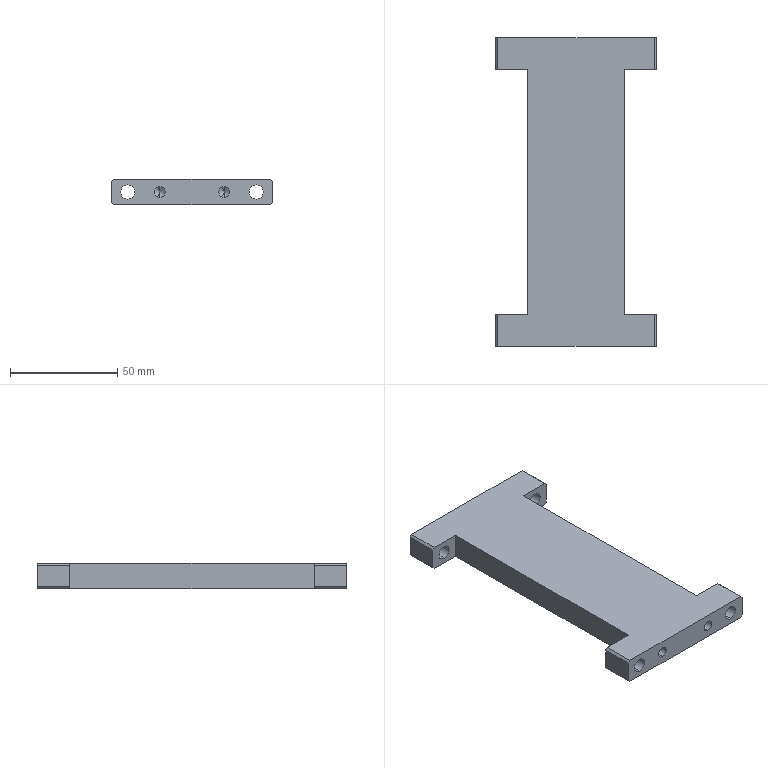Part | SolidWorks | features HoleWzd 2, MirrorPattern 2, Chamfer 1, Extrusion 1, ICE 1 | 1 solid | 46 faces | box 75 x 144 x 12 mm | volume 85544 mm3 | plane 22 | cylinder 16 | cone 8 | commonest cylinder face diameters 5 x8 6.6 x8
STEP:
#1=CARTESIAN_POINT('',(15.,61.,-2.5));
#2=VERTEX_POINT('',#1);
#3=CARTESIAN_POINT('',(15.,61.,2.5));
#4=VERTEX_POINT('',#3);
#5=CARTESIAN_POINT('',(15.,61.,0.));
#6=DIRECTION('',(0.,1.,0.));
#7=DIRECTION('',(0.,0.,1.));
#8=AXIS2_PLACEMENT_3D('',#5,#6,#7);
#9=CIRCLE('',#8,2.5);
#10=EDGE_CURVE('',#2,#4,#9,.T.);
#11=ORIENTED_EDGE('',*,*,#10,.F.);
#12=CARTESIAN_POINT('',(15.,72.,-2.5));
#13=VERTEX_POINT('',#12);
#14=CARTESIAN_POINT('',(15.,72.,-2.5));
#15=DIRECTION('',(0.,1.,0.));
#16=VECTOR('',#15,1000.);
#17=LINE('',#14,#16);
#18=EDGE_CURVE('',#2,#13,#17,.T.);
#19=ORIENTED_EDGE('',*,*,#18,.T.);
#20=CARTESIAN_POINT('',(15.,72.,2.5));
#21=VERTEX_POINT('',#20);
#22=CARTESIAN_POINT('',(15.,72.,0.));
#23=DIRECTION('',(0.,1.,0.));
#24=DIRECTION('',(0.,0.,1.));
#25=AXIS2_PLACEMENT_3D('',#22,#23,#24);
#26=CIRCLE('',#25,2.5);
#27=EDGE_CURVE('',#13,#21,#26,.T.);
#28=ORIENTED_EDGE('',*,*,#27,.T.);
#29=CARTESIAN_POINT('',(15.,72.,2.5));
#30=DIRECTION('',(0.,1.,0.));
#31=VECTOR('',#30,1000.);
#32=LINE('',#29,#31);
#33=EDGE_CURVE('',#4,#21,#32,.T.);
#34=ORIENTED_EDGE('',*,*,#33,.F.);
#35=EDGE_LOOP('',(#11,#19,#28,#34));
#36=FACE_OUTER_BOUND('',#35,.T.);
#37=CARTESIAN_POINT('',(15.,72.,0.));
#38=DIRECTION('',(0.,1.,0.));
#39=DIRECTION('',(0.,0.,1.));
#40=AXIS2_PLACEMENT_3D('',#37,#38,#39);
#41=CYLINDRICAL_SURFACE('',#40,2.5);
#42=ADVANCED_FACE('',(#36),#41,.F.);
#43=CARTESIAN_POINT('',(15.,59.498,0.));
#44=VERTEX_POINT('',#43);
#45=CARTESIAN_POINT('',(15.,61.,2.5));
#46=DIRECTION('',(0.,0.515,0.8572));
#47=VECTOR('',#46,1000.);
#48=LINE('',#45,#47);
#49=EDGE_CURVE('',#44,#4,#48,.T.);
#50=ORIENTED_EDGE('',*,*,#49,.F.);
#51=CARTESIAN_POINT('',(15.,61.,-2.5));
#52=DIRECTION('',(0.,0.515,-0.8572));
#53=VECTOR('',#52,1000.);
#54=LINE('',#51,#53);
#55=EDGE_CURVE('',#44,#2,#54,.T.);
#56=ORIENTED_EDGE('',*,*,#55,.T.);
#57=ORIENTED_EDGE('',*,*,#10,.T.);
#58=EDGE_LOOP('',(#50,#56,#57));
#59=FACE_OUTER_BOUND('',#58,.T.);
#60=CARTESIAN_POINT('',(15.,61.,0.));
#61=DIRECTION('',(0.,1.,0.));
#62=DIRECTION('',(0.,0.,1.));
#63=AXIS2_PLACEMENT_3D('',#60,#61,#62);
#64=CONICAL_SURFACE('',#63,2.5,1.03);
#65=ADVANCED_FACE('',(#59),#64,.F.);
#66=CARTESIAN_POINT('',(-15.,61.,-2.5));
#67=VERTEX_POINT('',#66);
#68=CARTESIAN_POINT('',(-15.,61.,2.5));
#69=VERTEX_POINT('',#68);
#70=CARTESIAN_POINT('',(-15.,61.,0.));
#71=DIRECTION('',(0.,1.,0.));
#72=DIRECTION('',(0.,0.,1.));
#73=AXIS2_PLACEMENT_3D('',#70,#71,#72);
#74=CIRCLE('',#73,2.5);
#75=EDGE_CURVE('',#67,#69,#74,.T.);
#76=ORIENTED_EDGE('',*,*,#75,.F.);
#77=CARTESIAN_POINT('',(-15.,72.,-2.5));
#78=VERTEX_POINT('',#77);
#79=CARTESIAN_POINT('',(-15.,72.,-2.5));
#80=DIRECTION('',(0.,1.,0.));
#81=VECTOR('',#80,1000.);
#82=LINE('',#79,#81);
#83=EDGE_CURVE('',#67,#78,#82,.T.);
#84=ORIENTED_EDGE('',*,*,#83,.T.);
#85=CARTESIAN_POINT('',(-15.,72.,2.5));
#86=VERTEX_POINT('',#85);
#87=CARTESIAN_POINT('',(-15.,72.,0.));
#88=DIRECTION('',(0.,1.,0.));
#89=DIRECTION('',(0.,0.,1.));
#90=AXIS2_PLACEMENT_3D('',#87,#88,#89);
#91=CIRCLE('',#90,2.5);
#92=EDGE_CURVE('',#78,#86,#91,.T.);
#93=ORIENTED_EDGE('',*,*,#92,.T.);
#94=CARTESIAN_POINT('',(-15.,72.,2.5));
#95=DIRECTION('',(0.,1.,0.));
#96=VECTOR('',#95,1000.);
#97=LINE('',#94,#96);
#98=EDGE_CURVE('',#69,#86,#97,.T.);
#99=ORIENTED_EDGE('',*,*,#98,.F.);
#100=EDGE_LOOP('',(#76,#84,#93,#99));
#101=FACE_OUTER_BOUND('',#100,.T.);
#102=CARTESIAN_POINT('',(-15.,72.,0.));
#103=DIRECTION('',(0.,1.,0.));
#104=DIRECTION('',(0.,0.,1.));
#105=AXIS2_PLACEMENT_3D('',#102,#103,#104);
#106=CYLINDRICAL_SURFACE('',#105,2.5);
#107=ADVANCED_FACE('',(#101),#106,.F.);
#108=CARTESIAN_POINT('',(-15.,59.498,0.));
#109=VERTEX_POINT('',#108);
#110=CARTESIAN_POINT('',(-15.,61.,2.5));
#111=DIRECTION('',(0.,0.515,0.8572));
#112=VECTOR('',#111,1000.);
#113=LINE('',#110,#112);
#114=EDGE_CURVE('',#109,#69,#113,.T.);
#115=ORIENTED_EDGE('',*,*,#114,.F.);
#116=CARTESIAN_POINT('',(-15.,61.,-2.5));
#117=DIRECTION('',(0.,0.515,-0.8572));
#118=VECTOR('',#117,1000.);
#119=LINE('',#116,#118);
#120=EDGE_CURVE('',#109,#67,#119,.T.);
#121=ORIENTED_EDGE('',*,*,#120,.T.);
#122=ORIENTED_EDGE('',*,*,#75,.T.);
#123=EDGE_LOOP('',(#115,#121,#122));
#124=FACE_OUTER_BOUND('',#123,.T.);
#125=CARTESIAN_POINT('',(-15.,61.,0.));
#126=DIRECTION('',(0.,1.,0.));
#127=DIRECTION('',(0.,0.,1.));
#128=AXIS2_PLACEMENT_3D('',#125,#126,#127);
#129=CONICAL_SURFACE('',#128,2.5,1.03);
#130=ADVANCED_FACE('',(#124),#129,.F.);
#131=CARTESIAN_POINT('',(15.,-61.,2.5));
#132=VERTEX_POINT('',#131);
#133=CARTESIAN_POINT('',(15.,-61.,-2.5));
#134=VERTEX_POINT('',#133);
#135=CARTESIAN_POINT('',(15.,-61.,0.));
#136=DIRECTION('',(0.,-1.,0.));
#137=DIRECTION('',(0.,0.,-1.));
#138=AXIS2_PLACEMENT_3D('',#135,#136,#137);
#139=CIRCLE('',#138,2.5);
#140=EDGE_CURVE('',#132,#134,#139,.T.);
#141=ORIENTED_EDGE('',*,*,#140,.F.);
#142=CARTESIAN_POINT('',(15.,-72.,2.5));
#143=VERTEX_POINT('',#142);
#144=CARTESIAN_POINT('',(15.,-72.,2.5));
#145=DIRECTION('',(0.,-1.,0.));
#146=VECTOR('',#145,1000.);
#147=LINE('',#144,#146);
#148=EDGE_CURVE('',#132,#143,#147,.T.);
#149=ORIENTED_EDGE('',*,*,#148,.T.);
#150=CARTESIAN_POINT('',(15.,-72.,-2.5));
#151=VERTEX_POINT('',#150);
#152=CARTESIAN_POINT('',(15.,-72.,0.));
#153=DIRECTION('',(0.,-1.,0.));
#154=DIRECTION('',(0.,0.,-1.));
#155=AXIS2_PLACEMENT_3D('',#152,#153,#154);
#156=CIRCLE('',#155,2.5);
#157=EDGE_CURVE('',#143,#151,#156,.T.);
#158=ORIENTED_EDGE('',*,*,#157,.T.);
#159=CARTESIAN_POINT('',(15.,-72.,-2.5));
#160=DIRECTION('',(0.,-1.,0.));
#161=VECTOR('',#160,1000.);
#162=LINE('',#159,#161);
#163=EDGE_CURVE('',#134,#151,#162,.T.);
#164=ORIENTED_EDGE('',*,*,#163,.F.);
#165=EDGE_LOOP('',(#141,#149,#158,#164));
#166=FACE_OUTER_BOUND('',#165,.T.);
#167=CARTESIAN_POINT('',(15.,-72.,0.));
#168=DIRECTION('',(0.,-1.,0.));
#169=DIRECTION('',(0.,0.,-1.));
#170=AXIS2_PLACEMENT_3D('',#167,#168,#169);
#171=CYLINDRICAL_SURFACE('',#170,2.5);
#172=ADVANCED_FACE('',(#166),#171,.F.);
#173=CARTESIAN_POINT('',(15.,-59.498,0.));
#174=VERTEX_POINT('',#173);
#175=CARTESIAN_POINT('',(15.,-61.,-2.5));
#176=DIRECTION('',(0.,-0.515,-0.8572));
#177=VECTOR('',#176,1000.);
#178=LINE('',#175,#177);
#179=EDGE_CURVE('',#174,#134,#178,.T.);
#180=ORIENTED_EDGE('',*,*,#179,.F.);
#181=CARTESIAN_POINT('',(15.,-61.,2.5));
#182=DIRECTION('',(0.,-0.515,0.8572));
#183=VECTOR('',#182,1000.);
#184=LINE('',#181,#183);
#185=EDGE_CURVE('',#174,#132,#184,.T.);
#186=ORIENTED_EDGE('',*,*,#185,.T.);
#187=ORIENTED_EDGE('',*,*,#140,.T.);
#188=EDGE_LOOP('',(#180,#186,#187));
#189=FACE_OUTER_BOUND('',#188,.T.);
#190=CARTESIAN_POINT('',(15.,-61.,0.));
#191=DIRECTION('',(0.,-1.,0.));
#192=DIRECTION('',(0.,0.,-1.));
#193=AXIS2_PLACEMENT_3D('',#190,#191,#192);
#194=CONICAL_SURFACE('',#193,2.5,1.03);
#195=ADVANCED_FACE('',(#189),#194,.F.);
#196=CARTESIAN_POINT('',(-15.,-61.,2.5));
#197=VERTEX_POINT('',#196);
#198=CARTESIAN_POINT('',(-15.,-61.,-2.5));
#199=VERTEX_POINT('',#198);
#200=CARTESIAN_POINT('',(-15.,-61.,0.));
#201=DIRECTION('',(0.,-1.,0.));
#202=DIRECTION('',(0.,0.,-1.));
#203=AXIS2_PLACEMENT_3D('',#200,#201,#202);
#204=CIRCLE('',#203,2.5);
#205=EDGE_CURVE('',#197,#199,#204,.T.);
#206=ORIENTED_EDGE('',*,*,#205,.F.);
#207=CARTESIAN_POINT('',(-15.,-72.,2.5));
#208=VERTEX_POINT('',#207);
#209=CARTESIAN_POINT('',(-15.,-72.,2.5));
#210=DIRECTION('',(0.,-1.,0.));
#211=VECTOR('',#210,1000.);
#212=LINE('',#209,#211);
#213=EDGE_CURVE('',#197,#208,#212,.T.);
#214=ORIENTED_EDGE('',*,*,#213,.T.);
#215=CARTESIAN_POINT('',(-15.,-72.,-2.5));
#216=VERTEX_POINT('',#215);
#217=CARTESIAN_POINT('',(-15.,-72.,0.));
#218=DIRECTION('',(0.,-1.,0.));
#219=DIRECTION('',(0.,0.,-1.));
#220=AXIS2_PLACEMENT_3D('',#217,#218,#219);
#221=CIRCLE('',#220,2.5);
#222=EDGE_CURVE('',#208,#216,#221,.T.);
#223=ORIENTED_EDGE('',*,*,#222,.T.);
#224=CARTESIAN_POINT('',(-15.,-72.,-2.5));
#225=DIRECTION('',(0.,-1.,0.));
#226=VECTOR('',#225,1000.);
#227=LINE('',#224,#226);
#228=EDGE_CURVE('',#199,#216,#227,.T.);
#229=ORIENTED_EDGE('',*,*,#228,.F.);
#230=EDGE_LOOP('',(#206,#214,#223,#229));
#231=FACE_OUTER_BOUND('',#230,.T.);
#232=CARTESIAN_POINT('',(-15.,-72.,0.));
#233=DIRECTION('',(0.,-1.,0.));
#234=DIRECTION('',(0.,0.,-1.));
#235=AXIS2_PLACEMENT_3D('',#232,#233,#234);
#236=CYLINDRICAL_SURFACE('',#235,2.5);
#237=ADVANCED_FACE('',(#231),#236,.F.);
#238=CARTESIAN_POINT('',(-15.,-59.498,0.));
#239=VERTEX_POINT('',#238);
#240=CARTESIAN_POINT('',(-15.,-61.,-2.5));
#241=DIRECTION('',(0.,-0.515,-0.8572));
#242=VECTOR('',#241,1000.);
#243=LINE('',#240,#242);
#244=EDGE_CURVE('',#239,#199,#243,.T.);
#245=ORIENTED_EDGE('',*,*,#244,.F.);
#246=CARTESIAN_POINT('',(-15.,-61.,2.5));
#247=DIRECTION('',(0.,-0.515,0.8572));
#248=VECTOR('',#247,1000.);
#249=LINE('',#246,#248);
#250=EDGE_CURVE('',#239,#197,#249,.T.);
#251=ORIENTED_EDGE('',*,*,#250,.T.);
#252=ORIENTED_EDGE('',*,*,#205,.T.);
#253=EDGE_LOOP('',(#245,#251,#252));
#254=FACE_OUTER_BOUND('',#253,.T.);
#255=CARTESIAN_POINT('',(-15.,-61.,0.));
#256=DIRECTION('',(0.,-1.,0.));
#257=DIRECTION('',(0.,0.,-1.));
#258=AXIS2_PLACEMENT_3D('',#255,#256,#257);
#259=CONICAL_SURFACE('',#258,2.5,1.03);
#260=ADVANCED_FACE('',(#254),#259,.F.);
#261=CARTESIAN_POINT('',(30.,72.,3.3));
#262=VERTEX_POINT('',#261);
#263=CARTESIAN_POINT('',(30.,72.,-3.3));
#264=VERTEX_POINT('',#263);
#265=CARTESIAN_POINT('',(30.,72.,0.));
#266=DIRECTION('',(0.,-1.,0.));
#267=DIRECTION('',(0.,0.,-1.));
#268=AXIS2_PLACEMENT_3D('',#265,#266,#267);
#269=CIRCLE('',#268,3.3);
#270=EDGE_CURVE('',#262,#264,#269,.T.);
#271=ORIENTED_EDGE('',*,*,#270,.F.);
#272=CARTESIAN_POINT('',(30.,57.,3.3));
#273=VERTEX_POINT('',#272);
#274=CARTESIAN_POINT('',(30.,-72.,3.3));
#275=DIRECTION('',(0.,-1.,0.));
#276=VECTOR('',#275,1000.);
#277=LINE('',#274,#276);
#278=EDGE_CURVE('',#262,#273,#277,.T.);
#279=ORIENTED_EDGE('',*,*,#278,.T.);
#280=CARTESIAN_POINT('',(30.,57.,-3.3));
#281=VERTEX_POINT('',#280);
#282=CARTESIAN_POINT('',(30.,57.,0.));
#283=DIRECTION('',(0.,-1.,0.));
#284=DIRECTION('',(0.,0.,-1.));
#285=AXIS2_PLACEMENT_3D('',#282,#283,#284);
#286=CIRCLE('',#285,3.3);
#287=EDGE_CURVE('',#273,#281,#286,.T.);
#288=ORIENTED_EDGE('',*,*,#287,.T.);
#289=CARTESIAN_POINT('',(30.,-72.,-3.3));
#290=DIRECTION('',(0.,-1.,0.));
#291=VECTOR('',#290,1000.);
#292=LINE('',#289,#291);
#293=EDGE_CURVE('',#264,#281,#292,.T.);
#294=ORIENTED_EDGE('',*,*,#293,.F.);
#295=EDGE_LOOP('',(#271,#279,#288,#294));
#296=FACE_OUTER_BOUND('',#295,.T.);
#297=CARTESIAN_POINT('',(30.,-72.,0.));
#298=DIRECTION('',(0.,-1.,0.));
#299=DIRECTION('',(0.,0.,-1.));
#300=AXIS2_PLACEMENT_3D('',#297,#298,#299);
#301=CYLINDRICAL_SURFACE('',#300,3.3);
#302=ADVANCED_FACE('',(#296),#301,.F.);
#303=CARTESIAN_POINT('',(30.,-57.,-3.3));
#304=VERTEX_POINT('',#303);
#305=CARTESIAN_POINT('',(30.,-57.,3.3));
#306=VERTEX_POINT('',#305);
#307=CARTESIAN_POINT('',(30.,-57.,0.));
#308=DIRECTION('',(0.,1.,0.));
#309=DIRECTION('',(0.,0.,1.));
#310=AXIS2_PLACEMENT_3D('',#307,#308,#309);
#311=CIRCLE('',#310,3.3);
#312=EDGE_CURVE('',#304,#306,#311,.T.);
#313=ORIENTED_EDGE('',*,*,#312,.T.);
#314=CARTESIAN_POINT('',(30.,-72.,3.3));
#315=VERTEX_POINT('',#314);
#316=CARTESIAN_POINT('',(30.,-72.,3.3));
#317=DIRECTION('',(0.,-1.,0.));
#318=VECTOR('',#317,1000.);
#319=LINE('',#316,#318);
#320=EDGE_CURVE('',#306,#315,#319,.T.);
#321=ORIENTED_EDGE('',*,*,#320,.T.);
#322=CARTESIAN_POINT('',(30.,-72.,-3.3));
#323=VERTEX_POINT('',#322);
#324=CARTESIAN_POINT('',(30.,-72.,0.));
#325=DIRECTION('',(0.,-1.,0.));
#326=DIRECTION('',(0.,0.,-1.));
#327=AXIS2_PLACEMENT_3D('',#324,#325,#326);
#328=CIRCLE('',#327,3.3);
#329=EDGE_CURVE('',#315,#323,#328,.T.);
#330=ORIENTED_EDGE('',*,*,#329,.T.);
#331=CARTESIAN_POINT('',(30.,-72.,-3.3));
#332=DIRECTION('',(0.,-1.,0.));
#333=VECTOR('',#332,1000.);
#334=LINE('',#331,#333);
#335=EDGE_CURVE('',#304,#323,#334,.T.);
#336=ORIENTED_EDGE('',*,*,#335,.F.);
#337=EDGE_LOOP('',(#313,#321,#330,#336));
#338=FACE_OUTER_BOUND('',#337,.T.);
#339=CARTESIAN_POINT('',(30.,-72.,0.));
#340=DIRECTION('',(0.,-1.,0.));
#341=DIRECTION('',(0.,0.,-1.));
#342=AXIS2_PLACEMENT_3D('',#339,#340,#341);
#343=CYLINDRICAL_SURFACE('',#342,3.3);
#344=ADVANCED_FACE('',(#338),#343,.F.);
#345=CARTESIAN_POINT('',(-30.,-57.,3.3));
#346=VERTEX_POINT('',#345);
#347=CARTESIAN_POINT('',(-30.,-57.,-3.3));
#348=VERTEX_POINT('',#347);
#349=CARTESIAN_POINT('',(-30.,-57.,0.));
#350=DIRECTION('',(0.,-1.,0.));
#351=DIRECTION('',(0.,0.,-1.));
#352=AXIS2_PLACEMENT_3D('',#349,#350,#351);
#353=CIRCLE('',#352,3.3);
#354=EDGE_CURVE('',#346,#348,#353,.T.);
#355=ORIENTED_EDGE('',*,*,#354,.F.);
#356=CARTESIAN_POINT('',(-30.,-72.,3.3));
#357=VERTEX_POINT('',#356);
#358=CARTESIAN_POINT('',(-30.,-72.,3.3));
#359=DIRECTION('',(0.,-1.,0.));
#360=VECTOR('',#359,1000.);
#361=LINE('',#358,#360);
#362=EDGE_CURVE('',#346,#357,#361,.T.);
#363=ORIENTED_EDGE('',*,*,#362,.T.);
#364=CARTESIAN_POINT('',(-30.,-72.,-3.3));
#365=VERTEX_POINT('',#364);
#366=CARTESIAN_POINT('',(-30.,-72.,0.));
#367=DIRECTION('',(0.,-1.,0.));
#368=DIRECTION('',(0.,0.,-1.));
#369=AXIS2_PLACEMENT_3D('',#366,#367,#368);
#370=CIRCLE('',#369,3.3);
#371=EDGE_CURVE('',#357,#365,#370,.T.);
#372=ORIENTED_EDGE('',*,*,#371,.T.);
#373=CARTESIAN_POINT('',(-30.,-72.,-3.3));
#374=DIRECTION('',(0.,-1.,0.));
#375=VECTOR('',#374,1000.);
#376=LINE('',#373,#375);
#377=EDGE_CURVE('',#348,#365,#376,.T.);
#378=ORIENTED_EDGE('',*,*,#377,.F.);
#379=EDGE_LOOP('',(#355,#363,#372,#378));
#380=FACE_OUTER_BOUND('',#379,.T.);
#381=CARTESIAN_POINT('',(-30.,-72.,0.));
#382=DIRECTION('',(0.,-1.,0.));
#383=DIRECTION('',(0.,0.,-1.));
#384=AXIS2_PLACEMENT_3D('',#381,#382,#383);
#385=CYLINDRICAL_SURFACE('',#384,3.3);
#386=ADVANCED_FACE('',(#380),#385,.F.);
#387=CARTESIAN_POINT('',(-30.,72.,3.3));
#388=VERTEX_POINT('',#387);
#389=CARTESIAN_POINT('',(-30.,72.,-3.3));
#390=VERTEX_POINT('',#389);
#391=CARTESIAN_POINT('',(-30.,72.,0.));
#392=DIRECTION('',(0.,-1.,0.));
#393=DIRECTION('',(0.,0.,-1.));
#394=AXIS2_PLACEMENT_3D('',#391,#392,#393);
#395=CIRCLE('',#394,3.3);
#396=EDGE_CURVE('',#388,#390,#395,.T.);
#397=ORIENTED_EDGE('',*,*,#396,.F.);
#398=CARTESIAN_POINT('',(-30.,57.,3.3));
#399=VERTEX_POINT('',#398);
#400=CARTESIAN_POINT('',(-30.,-72.,3.3));
#401=DIRECTION('',(0.,-1.,0.));
#402=VECTOR('',#401,1000.);
#403=LINE('',#400,#402);
#404=EDGE_CURVE('',#388,#399,#403,.T.);
#405=ORIENTED_EDGE('',*,*,#404,.T.);
#406=CARTESIAN_POINT('',(-30.,57.,-3.3));
#407=VERTEX_POINT('',#406);
#408=CARTESIAN_POINT('',(-30.,57.,0.));
#409=DIRECTION('',(0.,1.,0.));
#410=DIRECTION('',(0.,0.,1.));
#411=AXIS2_PLACEMENT_3D('',#408,#409,#410);
#412=CIRCLE('',#411,3.3);
#413=EDGE_CURVE('',#407,#399,#412,.T.);
#414=ORIENTED_EDGE('',*,*,#413,.F.);
#415=CARTESIAN_POINT('',(-30.,-72.,-3.3));
#416=DIRECTION('',(0.,-1.,0.));
#417=VECTOR('',#416,1000.);
#418=LINE('',#415,#417);
#419=EDGE_CURVE('',#390,#407,#418,.T.);
#420=ORIENTED_EDGE('',*,*,#419,.F.);
#421=EDGE_LOOP('',(#397,#405,#414,#420));
#422=FACE_OUTER_BOUND('',#421,.T.);
#423=CARTESIAN_POINT('',(-30.,-72.,0.));
#424=DIRECTION('',(0.,-1.,0.));
#425=DIRECTION('',(0.,0.,-1.));
#426=AXIS2_PLACEMENT_3D('',#423,#424,#425);
#427=CYLINDRICAL_SURFACE('',#426,3.3);
#428=ADVANCED_FACE('',(#422),#427,.F.);
#429=CARTESIAN_POINT('',(37.5,72.,5.));
#430=VERTEX_POINT('',#429);
#431=CARTESIAN_POINT('',(37.5,72.,-5.));
#432=VERTEX_POINT('',#431);
#433=CARTESIAN_POINT('',(37.5,72.,6.));
#434=DIRECTION('',(0.,0.,-1.));
#435=VECTOR('',#434,1000.);
#436=LINE('',#433,#435);
#437=EDGE_CURVE('',#430,#432,#436,.T.);
#438=ORIENTED_EDGE('',*,*,#437,.F.);
#439=CARTESIAN_POINT('',(37.5,57.,5.));
#440=VERTEX_POINT('',#439);
#441=CARTESIAN_POINT('',(37.5,57.,5.));
#442=DIRECTION('',(0.,-1.,0.));
#443=VECTOR('',#442,1000.);
#444=LINE('',#441,#443);
#445=EDGE_CURVE('',#430,#440,#444,.T.);
#446=ORIENTED_EDGE('',*,*,#445,.T.);
#447=CARTESIAN_POINT('',(37.5,57.,-5.));
#448=VERTEX_POINT('',#447);
#449=CARTESIAN_POINT('',(37.5,57.,-6.));
#450=DIRECTION('',(0.,0.,1.));
#451=VECTOR('',#450,1000.);
#452=LINE('',#449,#451);
#453=EDGE_CURVE('',#448,#440,#452,.T.);
#454=ORIENTED_EDGE('',*,*,#453,.F.);
#455=CARTESIAN_POINT('',(37.5,72.,-5.));
#456=DIRECTION('',(0.,1.,0.));
#457=VECTOR('',#456,1000.);
#458=LINE('',#455,#457);
#459=EDGE_CURVE('',#448,#432,#458,.T.);
#460=ORIENTED_EDGE('',*,*,#459,.T.);
#461=EDGE_LOOP('',(#438,#446,#454,#460));
#462=FACE_OUTER_BOUND('',#461,.T.);
#463=CARTESIAN_POINT('',(37.5,72.,6.));
#464=DIRECTION('',(-1.,0.,0.));
#465=DIRECTION('',(0.,-1.,0.));
#466=AXIS2_PLACEMENT_3D('',#463,#464,#465);
#467=PLANE('',#466);
#468=ADVANCED_FACE('',(#462),#467,.F.);
#469=CARTESIAN_POINT('',(37.5,-72.,5.));
#470=VERTEX_POINT('',#469);
#471=CARTESIAN_POINT('',(37.5,-72.,-5.));
#472=VERTEX_POINT('',#471);
#473=CARTESIAN_POINT('',(37.5,-72.,6.));
#474=DIRECTION('',(0.,0.,-1.));
#475=VECTOR('',#474,1000.);
#476=LINE('',#473,#475);
#477=EDGE_CURVE('',#470,#472,#476,.T.);
#478=ORIENTED_EDGE('',*,*,#477,.T.);
#479=CARTESIAN_POINT('',(37.5,-57.,-5.));
#480=VERTEX_POINT('',#479);
#481=CARTESIAN_POINT('',(37.5,72.,-5.));
#482=DIRECTION('',(0.,1.,0.));
#483=VECTOR('',#482,1000.);
#484=LINE('',#481,#483);
#485=EDGE_CURVE('',#472,#480,#484,.T.);
#486=ORIENTED_EDGE('',*,*,#485,.T.);
#487=CARTESIAN_POINT('',(37.5,-57.,5.));
#488=VERTEX_POINT('',#487);
#489=CARTESIAN_POINT('',(37.5,-57.,-6.));
#490=DIRECTION('',(0.,0.,1.));
#491=VECTOR('',#490,1000.);
#492=LINE('',#489,#491);
#493=EDGE_CURVE('',#480,#488,#492,.T.);
#494=ORIENTED_EDGE('',*,*,#493,.T.);
#495=CARTESIAN_POINT('',(37.5,-72.,5.));
#496=DIRECTION('',(0.,-1.,0.));
#497=VECTOR('',#496,1000.);
#498=LINE('',#495,#497);
#499=EDGE_CURVE('',#488,#470,#498,.T.);
#500=ORIENTED_EDGE('',*,*,#499,.T.);
#501=EDGE_LOOP('',(#478,#486,#494,#500));
#502=FACE_OUTER_BOUND('',#501,.T.);
#503=CARTESIAN_POINT('',(37.5,72.,6.));
#504=DIRECTION('',(-1.,0.,0.));
#505=DIRECTION('',(0.,-1.,0.));
#506=AXIS2_PLACEMENT_3D('',#503,#504,#505);
#507=PLANE('',#506);
#508=ADVANCED_FACE('',(#502),#507,.F.);
#509=CARTESIAN_POINT('',(-36.5,-72.,6.));
#510=VERTEX_POINT('',#509);
#511=CARTESIAN_POINT('',(36.5,-72.,6.));
#512=VERTEX_POINT('',#511);
#513=CARTESIAN_POINT('',(-37.5,-72.,6.));
#514=DIRECTION('',(1.,0.,0.));
#515=VECTOR('',#514,1000.);
#516=LINE('',#513,#515);
#517=EDGE_CURVE('',#510,#512,#516,.T.);
#518=ORIENTED_EDGE('',*,*,#517,.T.);
#519=CARTESIAN_POINT('',(36.5,-57.,6.));
#520=VERTEX_POINT('',#519);
#521=CARTESIAN_POINT('',(36.5,-57.,6.));
#522=DIRECTION('',(0.,1.,0.));
#523=VECTOR('',#522,1000.);
#524=LINE('',#521,#523);
#525=EDGE_CURVE('',#512,#520,#524,.T.);
#526=ORIENTED_EDGE('',*,*,#525,.T.);
#527=CARTESIAN_POINT('',(22.5,-57.,6.));
#528=VERTEX_POINT('',#527);
#529=CARTESIAN_POINT('',(37.5,-57.,6.));
#530=DIRECTION('',(-1.,0.,0.));
#531=VECTOR('',#530,1000.);
#532=LINE('',#529,#531);
#533=EDGE_CURVE('',#520,#528,#532,.T.);
#534=ORIENTED_EDGE('',*,*,#533,.T.);
#535=CARTESIAN_POINT('',(22.5,57.,6.));
#536=VERTEX_POINT('',#535);
#537=CARTESIAN_POINT('',(22.5,57.,6.));
#538=DIRECTION('',(0.,1.,0.));
#539=VECTOR('',#538,1000.);
#540=LINE('',#537,#539);
#541=EDGE_CURVE('',#528,#536,#540,.T.);
#542=ORIENTED_EDGE('',*,*,#541,.T.);
#543=CARTESIAN_POINT('',(36.5,57.,6.));
#544=VERTEX_POINT('',#543);
#545=CARTESIAN_POINT('',(37.5,57.,6.));
#546=DIRECTION('',(1.,0.,0.));
#547=VECTOR('',#546,1000.);
#548=LINE('',#545,#547);
#549=EDGE_CURVE('',#536,#544,#548,.T.);
#550=ORIENTED_EDGE('',*,*,#549,.T.);
#551=CARTESIAN_POINT('',(36.5,72.,6.));
#552=VERTEX_POINT('',#551);
#553=CARTESIAN_POINT('',(36.5,72.,6.));
#554=DIRECTION('',(0.,1.,0.));
#555=VECTOR('',#554,1000.);
#556=LINE('',#553,#555);
#557=EDGE_CURVE('',#544,#552,#556,.T.);
#558=ORIENTED_EDGE('',*,*,#557,.T.);
#559=CARTESIAN_POINT('',(-36.5,72.,6.));
#560=VERTEX_POINT('',#559);
#561=CARTESIAN_POINT('',(-37.5,72.,6.));
#562=DIRECTION('',(-1.,0.,0.));
#563=VECTOR('',#562,1000.);
#564=LINE('',#561,#563);
#565=EDGE_CURVE('',#552,#560,#564,.T.);
#566=ORIENTED_EDGE('',*,*,#565,.T.);
#567=CARTESIAN_POINT('',(-36.5,57.,6.));
#568=VERTEX_POINT('',#567);
#569=CARTESIAN_POINT('',(-36.5,57.,6.));
#570=DIRECTION('',(0.,-1.,0.));
#571=VECTOR('',#570,1000.);
#572=LINE('',#569,#571);
#573=EDGE_CURVE('',#560,#568,#572,.T.);
#574=ORIENTED_EDGE('',*,*,#573,.T.);
#575=CARTESIAN_POINT('',(-22.5,57.,6.));
#576=VERTEX_POINT('',#575);
#577=CARTESIAN_POINT('',(-37.5,57.,6.));
#578=DIRECTION('',(-1.,0.,0.));
#579=VECTOR('',#578,1000.);
#580=LINE('',#577,#579);
#581=EDGE_CURVE('',#576,#568,#580,.T.);
#582=ORIENTED_EDGE('',*,*,#581,.F.);
#583=CARTESIAN_POINT('',(-22.5,-57.,6.));
#584=VERTEX_POINT('',#583);
#585=CARTESIAN_POINT('',(-22.5,57.,6.));
#586=DIRECTION('',(0.,1.,0.));
#587=VECTOR('',#586,1000.);
#588=LINE('',#585,#587);
#589=EDGE_CURVE('',#584,#576,#588,.T.);
#590=ORIENTED_EDGE('',*,*,#589,.F.);
#591=CARTESIAN_POINT('',(-36.5,-57.,6.));
#592=VERTEX_POINT('',#591);
#593=CARTESIAN_POINT('',(-37.5,-57.,6.));
#594=DIRECTION('',(1.,0.,0.));
#595=VECTOR('',#594,1000.);
#596=LINE('',#593,#595);
#597=EDGE_CURVE('',#592,#584,#596,.T.);
#598=ORIENTED_EDGE('',*,*,#597,.F.);
#599=CARTESIAN_POINT('',(-36.5,-72.,6.));
#600=DIRECTION('',(0.,-1.,0.));
#601=VECTOR('',#600,1000.);
#602=LINE('',#599,#601);
#603=EDGE_CURVE('',#592,#510,#602,.T.);
#604=ORIENTED_EDGE('',*,*,#603,.T.);
#605=EDGE_LOOP('',(#518,#526,#534,#542,#550,#558,#566,#574,#582,#590,#598,#604));
#606=FACE_OUTER_BOUND('',#605,.T.);
#607=CARTESIAN_POINT('',(0.,0.,6.));
#608=DIRECTION('',(0.,0.,1.));
#609=DIRECTION('',(1.,0.,0.));
#610=AXIS2_PLACEMENT_3D('',#607,#608,#609);
#611=PLANE('',#610);
#612=ADVANCED_FACE('',(#606),#611,.T.);
#613=CARTESIAN_POINT('',(36.5,-57.,-6.));
#614=VERTEX_POINT('',#613);
#615=CARTESIAN_POINT('',(22.5,-57.,-6.));
#616=VERTEX_POINT('',#615);
#617=CARTESIAN_POINT('',(37.5,-57.,-6.));
#618=DIRECTION('',(-1.,0.,0.));
#619=VECTOR('',#618,1000.);
#620=LINE('',#617,#619);
#621=EDGE_CURVE('',#614,#616,#620,.T.);
#622=ORIENTED_EDGE('',*,*,#621,.F.);
#623=CARTESIAN_POINT('',(36.5,-72.,-6.));
#624=VERTEX_POINT('',#623);
#625=CARTESIAN_POINT('',(36.5,0.,-6.));
#626=DIRECTION('',(0.,-1.,0.));
#627=VECTOR('',#626,1000.);
#628=LINE('',#625,#627);
#629=EDGE_CURVE('',#614,#624,#628,.T.);
#630=ORIENTED_EDGE('',*,*,#629,.T.);
#631=CARTESIAN_POINT('',(-36.5,-72.,-6.));
#632=VERTEX_POINT('',#631);
#633=CARTESIAN_POINT('',(-37.5,-72.,-6.));
#634=DIRECTION('',(1.,0.,0.));
#635=VECTOR('',#634,1000.);
#636=LINE('',#633,#635);
#637=EDGE_CURVE('',#632,#624,#636,.T.);
#638=ORIENTED_EDGE('',*,*,#637,.F.);
#639=CARTESIAN_POINT('',(-36.5,-57.,-6.));
#640=VERTEX_POINT('',#639);
#641=CARTESIAN_POINT('',(-36.5,0.,-6.));
#642=DIRECTION('',(0.,1.,0.));
#643=VECTOR('',#642,1000.);
#644=LINE('',#641,#643);
#645=EDGE_CURVE('',#632,#640,#644,.T.);
#646=ORIENTED_EDGE('',*,*,#645,.T.);
#647=CARTESIAN_POINT('',(-22.5,-57.,-6.));
#648=VERTEX_POINT('',#647);
#649=CARTESIAN_POINT('',(-37.5,-57.,-6.));
#650=DIRECTION('',(1.,0.,0.));
#651=VECTOR('',#650,1000.);
#652=LINE('',#649,#651);
#653=EDGE_CURVE('',#640,#648,#652,.T.);
#654=ORIENTED_EDGE('',*,*,#653,.T.);
#655=CARTESIAN_POINT('',(-22.5,57.,-6.));
#656=VERTEX_POINT('',#655);
#657=CARTESIAN_POINT('',(-22.5,57.,-6.));
#658=DIRECTION('',(0.,1.,0.));
#659=VECTOR('',#658,1000.);
#660=LINE('',#657,#659);
#661=EDGE_CURVE('',#648,#656,#660,.T.);
#662=ORIENTED_EDGE('',*,*,#661,.T.);
#663=CARTESIAN_POINT('',(-36.5,57.,-6.));
#664=VERTEX_POINT('',#663);
#665=CARTESIAN_POINT('',(-37.5,57.,-6.));
#666=DIRECTION('',(-1.,0.,0.));
#667=VECTOR('',#666,1000.);
#668=LINE('',#665,#667);
#669=EDGE_CURVE('',#656,#664,#668,.T.);
#670=ORIENTED_EDGE('',*,*,#669,.T.);
#671=CARTESIAN_POINT('',(-36.5,72.,-6.));
#672=VERTEX_POINT('',#671);
#673=CARTESIAN_POINT('',(-36.5,0.,-6.));
#674=DIRECTION('',(0.,1.,0.));
#675=VECTOR('',#674,1000.);
#676=LINE('',#673,#675);
#677=EDGE_CURVE('',#664,#672,#676,.T.);
#678=ORIENTED_EDGE('',*,*,#677,.T.);
#679=CARTESIAN_POINT('',(36.5,72.,-6.));
#680=VERTEX_POINT('',#679);
#681=CARTESIAN_POINT('',(-37.5,72.,-6.));
#682=DIRECTION('',(-1.,0.,0.));
#683=VECTOR('',#682,1000.);
#684=LINE('',#681,#683);
#685=EDGE_CURVE('',#680,#672,#684,.T.);
#686=ORIENTED_EDGE('',*,*,#685,.F.);
#687=CARTESIAN_POINT('',(36.5,57.,-6.));
#688=VERTEX_POINT('',#687);
#689=CARTESIAN_POINT('',(36.5,0.,-6.));
#690=DIRECTION('',(0.,-1.,0.));
#691=VECTOR('',#690,1000.);
#692=LINE('',#689,#691);
#693=EDGE_CURVE('',#680,#688,#692,.T.);
#694=ORIENTED_EDGE('',*,*,#693,.T.);
#695=CARTESIAN_POINT('',(22.5,57.,-6.));
#696=VERTEX_POINT('',#695);
#697=CARTESIAN_POINT('',(37.5,57.,-6.));
#698=DIRECTION('',(1.,0.,0.));
#699=VECTOR('',#698,1000.);
#700=LINE('',#697,#699);
#701=EDGE_CURVE('',#696,#688,#700,.T.);
#702=ORIENTED_EDGE('',*,*,#701,.F.);
#703=CARTESIAN_POINT('',(22.5,57.,-6.));
#704=DIRECTION('',(0.,1.,0.));
#705=VECTOR('',#704,1000.);
#706=LINE('',#703,#705);
#707=EDGE_CURVE('',#616,#696,#706,.T.);
#708=ORIENTED_EDGE('',*,*,#707,.F.);
#709=EDGE_LOOP('',(#622,#630,#638,#646,#654,#662,#670,#678,#686,#694,#702,#708));
#710=FACE_OUTER_BOUND('',#709,.T.);
#711=CARTESIAN_POINT('',(0.,0.,-6.));
#712=DIRECTION('',(0.,0.,1.));
#713=DIRECTION('',(1.,0.,0.));
#714=AXIS2_PLACEMENT_3D('',#711,#712,#713);
#715=PLANE('',#714);
#716=ADVANCED_FACE('',(#710),#715,.F.);
#717=CARTESIAN_POINT('',(-37.5,-72.,5.));
#718=VERTEX_POINT('',#717);
#719=CARTESIAN_POINT('',(-37.5,-72.,-5.));
#720=VERTEX_POINT('',#719);
#721=CARTESIAN_POINT('',(-37.5,-72.,6.));
#722=DIRECTION('',(0.,0.,-1.));
#723=VECTOR('',#722,1000.);
#724=LINE('',#721,#723);
#725=EDGE_CURVE('',#718,#720,#724,.T.);
#726=ORIENTED_EDGE('',*,*,#725,.F.);
#727=CARTESIAN_POINT('',(-37.5,-57.,5.));
#728=VERTEX_POINT('',#727);
#729=CARTESIAN_POINT('',(-37.5,-57.,5.));
#730=DIRECTION('',(0.,1.,0.));
#731=VECTOR('',#730,1000.);
#732=LINE('',#729,#731);
#733=EDGE_CURVE('',#718,#728,#732,.T.);
#734=ORIENTED_EDGE('',*,*,#733,.T.);
#735=CARTESIAN_POINT('',(-37.5,-57.,-5.));
#736=VERTEX_POINT('',#735);
#737=CARTESIAN_POINT('',(-37.5,-57.,-6.));
#738=DIRECTION('',(0.,0.,1.));
#739=VECTOR('',#738,1000.);
#740=LINE('',#737,#739);
#741=EDGE_CURVE('',#736,#728,#740,.T.);
#742=ORIENTED_EDGE('',*,*,#741,.F.);
#743=CARTESIAN_POINT('',(-37.5,72.,-5.));
#744=DIRECTION('',(0.,-1.,0.));
#745=VECTOR('',#744,1000.);
#746=LINE('',#743,#745);
#747=EDGE_CURVE('',#736,#720,#746,.T.);
#748=ORIENTED_EDGE('',*,*,#747,.T.);
#749=EDGE_LOOP('',(#726,#734,#742,#748));
#750=FACE_OUTER_BOUND('',#749,.T.);
#751=CARTESIAN_POINT('',(-37.5,72.,6.));
#752=DIRECTION('',(1.,0.,0.));
#753=DIRECTION('',(0.,1.,0.));
#754=AXIS2_PLACEMENT_3D('',#751,#752,#753);
#755=PLANE('',#754);
#756=ADVANCED_FACE('',(#750),#755,.F.);
#757=CARTESIAN_POINT('',(15.,72.,0.));
#758=DIRECTION('',(0.,1.,0.));
#759=DIRECTION('',(0.,0.,1.));
#760=AXIS2_PLACEMENT_3D('',#757,#758,#759);
#761=CIRCLE('',#760,2.5);
#762=EDGE_CURVE('',#21,#13,#761,.T.);
#763=ORIENTED_EDGE('',*,*,#762,.F.);
#764=ORIENTED_EDGE('',*,*,#27,.F.);
#765=EDGE_LOOP('',(#763,#764));
#766=FACE_BOUND('',#765,.T.);
#767=CARTESIAN_POINT('',(-15.,72.,0.));
#768=DIRECTION('',(0.,1.,0.));
#769=DIRECTION('',(0.,0.,1.));
#770=AXIS2_PLACEMENT_3D('',#767,#768,#769);
#771=CIRCLE('',#770,2.5);
#772=EDGE_CURVE('',#86,#78,#771,.T.);
#773=ORIENTED_EDGE('',*,*,#772,.F.);
#774=ORIENTED_EDGE('',*,*,#92,.F.);
#775=EDGE_LOOP('',(#773,#774));
#776=FACE_BOUND('',#775,.T.);
#777=CARTESIAN_POINT('',(30.,72.,0.));
#778=DIRECTION('',(0.,-1.,0.));
#779=DIRECTION('',(0.,0.,-1.));
#780=AXIS2_PLACEMENT_3D('',#777,#778,#779);
#781=CIRCLE('',#780,3.3);
#782=EDGE_CURVE('',#264,#262,#781,.T.);
#783=ORIENTED_EDGE('',*,*,#782,.T.);
#784=ORIENTED_EDGE('',*,*,#270,.T.);
#785=EDGE_LOOP('',(#783,#784));
#786=FACE_BOUND('',#785,.T.);
#787=CARTESIAN_POINT('',(-30.,72.,0.));
#788=DIRECTION('',(0.,-1.,0.));
#789=DIRECTION('',(0.,0.,-1.));
#790=AXIS2_PLACEMENT_3D('',#787,#788,#789);
#791=CIRCLE('',#790,3.3);
#792=EDGE_CURVE('',#390,#388,#791,.T.);
#793=ORIENTED_EDGE('',*,*,#792,.T.);
#794=ORIENTED_EDGE('',*,*,#396,.T.);
#795=EDGE_LOOP('',(#793,#794));
#796=FACE_BOUND('',#795,.T.);
#797=ORIENTED_EDGE('',*,*,#685,.T.);
#798=CARTESIAN_POINT('',(-37.5,72.,-5.));
#799=VERTEX_POINT('',#798);
#800=CARTESIAN_POINT('',(-37.5,72.,-5.));
#801=DIRECTION('',(-0.7071,0.,0.7071));
#802=VECTOR('',#801,1000.);
#803=LINE('',#800,#802);
#804=EDGE_CURVE('',#672,#799,#803,.T.);
#805=ORIENTED_EDGE('',*,*,#804,.T.);
#806=CARTESIAN_POINT('',(-37.5,72.,5.));
#807=VERTEX_POINT('',#806);
#808=CARTESIAN_POINT('',(-37.5,72.,6.));
#809=DIRECTION('',(0.,0.,-1.));
#810=VECTOR('',#809,1000.);
#811=LINE('',#808,#810);
#812=EDGE_CURVE('',#807,#799,#811,.T.);
#813=ORIENTED_EDGE('',*,*,#812,.F.);
#814=CARTESIAN_POINT('',(-36.5,72.,6.));
#815=DIRECTION('',(0.7071,0.,0.7071));
#816=VECTOR('',#815,1000.);
#817=LINE('',#814,#816);
#818=EDGE_CURVE('',#807,#560,#817,.T.);
#819=ORIENTED_EDGE('',*,*,#818,.T.);
#820=ORIENTED_EDGE('',*,*,#565,.F.);
#821=CARTESIAN_POINT('',(36.5,72.,6.));
#822=DIRECTION('',(0.7071,0.,-0.7071));
#823=VECTOR('',#822,1000.);
#824=LINE('',#821,#823);
#825=EDGE_CURVE('',#552,#430,#824,.T.);
#826=ORIENTED_EDGE('',*,*,#825,.T.);
#827=ORIENTED_EDGE('',*,*,#437,.T.);
#828=CARTESIAN_POINT('',(37.5,72.,-5.));
#829=DIRECTION('',(-0.7071,0.,-0.7071));
#830=VECTOR('',#829,1000.);
#831=LINE('',#828,#830);
#832=EDGE_CURVE('',#432,#680,#831,.T.);
#833=ORIENTED_EDGE('',*,*,#832,.T.);
#834=EDGE_LOOP('',(#797,#805,#813,#819,#820,#826,#827,#833));
#835=FACE_OUTER_BOUND('',#834,.T.);
#836=CARTESIAN_POINT('',(-37.5,72.,6.));
#837=DIRECTION('',(0.,-1.,0.));
#838=DIRECTION('',(0.,0.,-1.));
#839=AXIS2_PLACEMENT_3D('',#836,#837,#838);
#840=PLANE('',#839);
#841=ADVANCED_FACE('',(#766,#776,#786,#796,#835),#840,.F.);
#842=ORIENTED_EDGE('',*,*,#812,.T.);
#843=CARTESIAN_POINT('',(-37.5,57.,-5.));
#844=VERTEX_POINT('',#843);
#845=CARTESIAN_POINT('',(-37.5,72.,-5.));
#846=DIRECTION('',(0.,-1.,0.));
#847=VECTOR('',#846,1000.);
#848=LINE('',#845,#847);
#849=EDGE_CURVE('',#799,#844,#848,.T.);
#850=ORIENTED_EDGE('',*,*,#849,.T.);
#851=CARTESIAN_POINT('',(-37.5,57.,5.));
#852=VERTEX_POINT('',#851);
#853=CARTESIAN_POINT('',(-37.5,57.,-6.));
#854=DIRECTION('',(0.,0.,1.));
#855=VECTOR('',#854,1000.);
#856=LINE('',#853,#855);
#857=EDGE_CURVE('',#844,#852,#856,.T.);
#858=ORIENTED_EDGE('',*,*,#857,.T.);
#859=CARTESIAN_POINT('',(-37.5,72.,5.));
#860=DIRECTION('',(0.,1.,0.));
#861=VECTOR('',#860,1000.);
#862=LINE('',#859,#861);
#863=EDGE_CURVE('',#852,#807,#862,.T.);
#864=ORIENTED_EDGE('',*,*,#863,.T.);
#865=EDGE_LOOP('',(#842,#850,#858,#864));
#866=FACE_OUTER_BOUND('',#865,.T.);
#867=CARTESIAN_POINT('',(-37.5,72.,6.));
#868=DIRECTION('',(1.,0.,0.));
#869=DIRECTION('',(0.,1.,0.));
#870=AXIS2_PLACEMENT_3D('',#867,#868,#869);
#871=PLANE('',#870);
#872=ADVANCED_FACE('',(#866),#871,.F.);
#873=CARTESIAN_POINT('',(15.,-72.,0.));
#874=DIRECTION('',(0.,-1.,0.));
#875=DIRECTION('',(0.,0.,-1.));
#876=AXIS2_PLACEMENT_3D('',#873,#874,#875);
#877=CIRCLE('',#876,2.5);
#878=EDGE_CURVE('',#151,#143,#877,.T.);
#879=ORIENTED_EDGE('',*,*,#878,.F.);
#880=ORIENTED_EDGE('',*,*,#157,.F.);
#881=EDGE_LOOP('',(#879,#880));
#882=FACE_BOUND('',#881,.T.);
#883=CARTESIAN_POINT('',(-15.,-72.,0.));
#884=DIRECTION('',(0.,-1.,0.));
#885=DIRECTION('',(0.,0.,-1.));
#886=AXIS2_PLACEMENT_3D('',#883,#884,#885);
#887=CIRCLE('',#886,2.5);
#888=EDGE_CURVE('',#216,#208,#887,.T.);
#889=ORIENTED_EDGE('',*,*,#888,.F.);
#890=ORIENTED_EDGE('',*,*,#222,.F.);
#891=EDGE_LOOP('',(#889,#890));
#892=FACE_BOUND('',#891,.T.);
#893=CARTESIAN_POINT('',(30.,-72.,0.));
#894=DIRECTION('',(0.,-1.,0.));
#895=DIRECTION('',(0.,0.,-1.));
#896=AXIS2_PLACEMENT_3D('',#893,#894,#895);
#897=CIRCLE('',#896,3.3);
#898=EDGE_CURVE('',#323,#315,#897,.T.);
#899=ORIENTED_EDGE('',*,*,#898,.F.);
#900=ORIENTED_EDGE('',*,*,#329,.F.);
#901=EDGE_LOOP('',(#899,#900));
#902=FACE_BOUND('',#901,.T.);
#903=CARTESIAN_POINT('',(-30.,-72.,0.));
#904=DIRECTION('',(0.,-1.,0.));
#905=DIRECTION('',(0.,0.,-1.));
#906=AXIS2_PLACEMENT_3D('',#903,#904,#905);
#907=CIRCLE('',#906,3.3);
#908=EDGE_CURVE('',#365,#357,#907,.T.);
#909=ORIENTED_EDGE('',*,*,#908,.F.);
#910=ORIENTED_EDGE('',*,*,#371,.F.);
#911=EDGE_LOOP('',(#909,#910));
#912=FACE_BOUND('',#911,.T.);
#913=ORIENTED_EDGE('',*,*,#637,.T.);
#914=CARTESIAN_POINT('',(37.5,-72.,-5.));
#915=DIRECTION('',(0.7071,0.,0.7071));
#916=VECTOR('',#915,1000.);
#917=LINE('',#914,#916);
#918=EDGE_CURVE('',#624,#472,#917,.T.);
#919=ORIENTED_EDGE('',*,*,#918,.T.);
#920=ORIENTED_EDGE('',*,*,#477,.F.);
#921=CARTESIAN_POINT('',(36.5,-72.,6.));
#922=DIRECTION('',(-0.7071,0.,0.7071));
#923=VECTOR('',#922,1000.);
#924=LINE('',#921,#923);
#925=EDGE_CURVE('',#470,#512,#924,.T.);
#926=ORIENTED_EDGE('',*,*,#925,.T.);
#927=ORIENTED_EDGE('',*,*,#517,.F.);
#928=CARTESIAN_POINT('',(-36.5,-72.,6.));
#929=DIRECTION('',(-0.7071,0.,-0.7071));
#930=VECTOR('',#929,1000.);
#931=LINE('',#928,#930);
#932=EDGE_CURVE('',#510,#718,#931,.T.);
#933=ORIENTED_EDGE('',*,*,#932,.T.);
#934=ORIENTED_EDGE('',*,*,#725,.T.);
#935=CARTESIAN_POINT('',(-37.5,-72.,-5.));
#936=DIRECTION('',(0.7071,0.,-0.7071));
#937=VECTOR('',#936,1000.);
#938=LINE('',#935,#937);
#939=EDGE_CURVE('',#720,#632,#938,.T.);
#940=ORIENTED_EDGE('',*,*,#939,.T.);
#941=EDGE_LOOP('',(#913,#919,#920,#926,#927,#933,#934,#940));
#942=FACE_OUTER_BOUND('',#941,.T.);
#943=CARTESIAN_POINT('',(-37.5,-72.,6.));
#944=DIRECTION('',(0.,1.,0.));
#945=DIRECTION('',(0.,0.,1.));
#946=AXIS2_PLACEMENT_3D('',#943,#944,#945);
#947=PLANE('',#946);
#948=ADVANCED_FACE('',(#882,#892,#902,#912,#942),#947,.F.);
#949=ORIENTED_EDGE('',*,*,#589,.T.);
#950=CARTESIAN_POINT('',(-22.5,57.,-6.));
#951=DIRECTION('',(0.,0.,1.));
#952=VECTOR('',#951,1000.);
#953=LINE('',#950,#952);
#954=EDGE_CURVE('',#656,#576,#953,.T.);
#955=ORIENTED_EDGE('',*,*,#954,.F.);
#956=ORIENTED_EDGE('',*,*,#661,.F.);
#957=CARTESIAN_POINT('',(-22.5,-57.,-6.));
#958=DIRECTION('',(0.,0.,1.));
#959=VECTOR('',#958,1000.);
#960=LINE('',#957,#959);
#961=EDGE_CURVE('',#648,#584,#960,.T.);
#962=ORIENTED_EDGE('',*,*,#961,.T.);
#963=EDGE_LOOP('',(#949,#955,#956,#962));
#964=FACE_OUTER_BOUND('',#963,.T.);
#965=CARTESIAN_POINT('',(-22.5,57.,-6.));
#966=DIRECTION('',(1.,0.,0.));
#967=DIRECTION('',(0.,1.,0.));
#968=AXIS2_PLACEMENT_3D('',#965,#966,#967);
#969=PLANE('',#968);
#970=ADVANCED_FACE('',(#964),#969,.F.);
#971=CARTESIAN_POINT('',(-30.,-57.,0.));
#972=DIRECTION('',(0.,-1.,0.));
#973=DIRECTION('',(0.,0.,-1.));
#974=AXIS2_PLACEMENT_3D('',#971,#972,#973);
#975=CIRCLE('',#974,3.3);
#976=EDGE_CURVE('',#348,#346,#975,.T.);
#977=ORIENTED_EDGE('',*,*,#976,.T.);
#978=ORIENTED_EDGE('',*,*,#354,.T.);
#979=EDGE_LOOP('',(#977,#978));
#980=FACE_BOUND('',#979,.T.);
#981=ORIENTED_EDGE('',*,*,#741,.T.);
#982=CARTESIAN_POINT('',(-36.5,-57.,6.));
#983=DIRECTION('',(0.7071,0.,0.7071));
#984=VECTOR('',#983,1000.);
#985=LINE('',#982,#984);
#986=EDGE_CURVE('',#728,#592,#985,.T.);
#987=ORIENTED_EDGE('',*,*,#986,.T.);
#988=ORIENTED_EDGE('',*,*,#597,.T.);
#989=ORIENTED_EDGE('',*,*,#961,.F.);
#990=ORIENTED_EDGE('',*,*,#653,.F.);
#991=CARTESIAN_POINT('',(-37.5,-57.,-5.));
#992=DIRECTION('',(-0.7071,0.,0.7071));
#993=VECTOR('',#992,1000.);
#994=LINE('',#991,#993);
#995=EDGE_CURVE('',#640,#736,#994,.T.);
#996=ORIENTED_EDGE('',*,*,#995,.T.);
#997=EDGE_LOOP('',(#981,#987,#988,#989,#990,#996));
#998=FACE_OUTER_BOUND('',#997,.T.);
#999=CARTESIAN_POINT('',(-37.5,-57.,-6.));
#1000=DIRECTION('',(0.,-1.,0.));
#1001=DIRECTION('',(0.,0.,-1.));
#1002=AXIS2_PLACEMENT_3D('',#999,#1000,#1001);
#1003=PLANE('',#1002);
#1004=ADVANCED_FACE('',(#980,#998),#1003,.F.);
#1005=ORIENTED_EDGE('',*,*,#413,.T.);
#1006=CARTESIAN_POINT('',(-30.,57.,0.));
#1007=DIRECTION('',(0.,1.,0.));
#1008=DIRECTION('',(0.,0.,1.));
#1009=AXIS2_PLACEMENT_3D('',#1006,#1007,#1008);
#1010=CIRCLE('',#1009,3.3);
#1011=EDGE_CURVE('',#399,#407,#1010,.T.);
#1012=ORIENTED_EDGE('',*,*,#1011,.T.);
#1013=EDGE_LOOP('',(#1005,#1012));
#1014=FACE_BOUND('',#1013,.T.);
#1015=ORIENTED_EDGE('',*,*,#857,.F.);
#1016=CARTESIAN_POINT('',(-37.5,57.,-5.));
#1017=DIRECTION('',(0.7071,0.,-0.7071));
#1018=VECTOR('',#1017,1000.);
#1019=LINE('',#1016,#1018);
#1020=EDGE_CURVE('',#844,#664,#1019,.T.);
#1021=ORIENTED_EDGE('',*,*,#1020,.T.);
#1022=ORIENTED_EDGE('',*,*,#669,.F.);
#1023=ORIENTED_EDGE('',*,*,#954,.T.);
#1024=ORIENTED_EDGE('',*,*,#581,.T.);
#1025=CARTESIAN_POINT('',(-36.5,57.,6.));
#1026=DIRECTION('',(-0.7071,0.,-0.7071));
#1027=VECTOR('',#1026,1000.);
#1028=LINE('',#1025,#1027);
#1029=EDGE_CURVE('',#568,#852,#1028,.T.);
#1030=ORIENTED_EDGE('',*,*,#1029,.T.);
#1031=EDGE_LOOP('',(#1015,#1021,#1022,#1023,#1024,#1030));
#1032=FACE_OUTER_BOUND('',#1031,.T.);
#1033=CARTESIAN_POINT('',(-37.5,57.,-6.));
#1034=DIRECTION('',(0.,1.,0.));
#1035=DIRECTION('',(0.,0.,1.));
#1036=AXIS2_PLACEMENT_3D('',#1033,#1034,#1035);
#1037=PLANE('',#1036);
#1038=ADVANCED_FACE('',(#1014,#1032),#1037,.F.);
#1039=ORIENTED_EDGE('',*,*,#541,.F.);
#1040=CARTESIAN_POINT('',(22.5,-57.,-6.));
#1041=DIRECTION('',(0.,0.,1.));
#1042=VECTOR('',#1041,1000.);
#1043=LINE('',#1040,#1042);
#1044=EDGE_CURVE('',#616,#528,#1043,.T.);
#1045=ORIENTED_EDGE('',*,*,#1044,.F.);
#1046=ORIENTED_EDGE('',*,*,#707,.T.);
#1047=CARTESIAN_POINT('',(22.5,57.,-6.));
#1048=DIRECTION('',(0.,0.,1.));
#1049=VECTOR('',#1048,1000.);
#1050=LINE('',#1047,#1049);
#1051=EDGE_CURVE('',#696,#536,#1050,.T.);
#1052=ORIENTED_EDGE('',*,*,#1051,.T.);
#1053=EDGE_LOOP('',(#1039,#1045,#1046,#1052));
#1054=FACE_OUTER_BOUND('',#1053,.T.);
#1055=CARTESIAN_POINT('',(22.5,57.,-6.));
#1056=DIRECTION('',(1.,0.,0.));
#1057=DIRECTION('',(0.,1.,0.));
#1058=AXIS2_PLACEMENT_3D('',#1055,#1056,#1057);
#1059=PLANE('',#1058);
#1060=ADVANCED_FACE('',(#1054),#1059,.T.);
#1061=CARTESIAN_POINT('',(30.,57.,0.));
#1062=DIRECTION('',(0.,-1.,0.));
#1063=DIRECTION('',(0.,0.,-1.));
#1064=AXIS2_PLACEMENT_3D('',#1061,#1062,#1063);
#1065=CIRCLE('',#1064,3.3);
#1066=EDGE_CURVE('',#281,#273,#1065,.T.);
#1067=ORIENTED_EDGE('',*,*,#1066,.F.);
#1068=ORIENTED_EDGE('',*,*,#287,.F.);
#1069=EDGE_LOOP('',(#1067,#1068));
#1070=FACE_BOUND('',#1069,.T.);
#1071=ORIENTED_EDGE('',*,*,#453,.T.);
#1072=CARTESIAN_POINT('',(43.,57.,-0.5));
#1073=DIRECTION('',(-0.7071,0.,0.7071));
#1074=VECTOR('',#1073,1000.);
#1075=LINE('',#1072,#1074);
#1076=EDGE_CURVE('',#440,#544,#1075,.T.);
#1077=ORIENTED_EDGE('',*,*,#1076,.T.);
#1078=ORIENTED_EDGE('',*,*,#549,.F.);
#1079=ORIENTED_EDGE('',*,*,#1051,.F.);
#1080=ORIENTED_EDGE('',*,*,#701,.T.);
#1081=CARTESIAN_POINT('',(37.,57.,-5.5));
#1082=DIRECTION('',(0.7071,0.,0.7071));
#1083=VECTOR('',#1082,1000.);
#1084=LINE('',#1081,#1083);
#1085=EDGE_CURVE('',#688,#448,#1084,.T.);
#1086=ORIENTED_EDGE('',*,*,#1085,.T.);
#1087=EDGE_LOOP('',(#1071,#1077,#1078,#1079,#1080,#1086));
#1088=FACE_OUTER_BOUND('',#1087,.T.);
#1089=CARTESIAN_POINT('',(37.5,57.,-6.));
#1090=DIRECTION('',(0.,-1.,0.));
#1091=DIRECTION('',(0.,0.,-1.));
#1092=AXIS2_PLACEMENT_3D('',#1089,#1090,#1091);
#1093=PLANE('',#1092);
#1094=ADVANCED_FACE('',(#1070,#1088),#1093,.T.);
#1095=ORIENTED_EDGE('',*,*,#312,.F.);
#1096=CARTESIAN_POINT('',(30.,-57.,0.));
#1097=DIRECTION('',(0.,1.,0.));
#1098=DIRECTION('',(0.,0.,1.));
#1099=AXIS2_PLACEMENT_3D('',#1096,#1097,#1098);
#1100=CIRCLE('',#1099,3.3);
#1101=EDGE_CURVE('',#306,#304,#1100,.T.);
#1102=ORIENTED_EDGE('',*,*,#1101,.F.);
#1103=EDGE_LOOP('',(#1095,#1102));
#1104=FACE_BOUND('',#1103,.T.);
#1105=ORIENTED_EDGE('',*,*,#493,.F.);
#1106=CARTESIAN_POINT('',(37.,-57.,-5.5));
#1107=DIRECTION('',(-0.7071,0.,-0.7071));
#1108=VECTOR('',#1107,1000.);
#1109=LINE('',#1106,#1108);
#1110=EDGE_CURVE('',#480,#614,#1109,.T.);
#1111=ORIENTED_EDGE('',*,*,#1110,.T.);
#1112=ORIENTED_EDGE('',*,*,#621,.T.);
#1113=ORIENTED_EDGE('',*,*,#1044,.T.);
#1114=ORIENTED_EDGE('',*,*,#533,.F.);
#1115=CARTESIAN_POINT('',(43.,-57.,-0.5));
#1116=DIRECTION('',(0.7071,0.,-0.7071));
#1117=VECTOR('',#1116,1000.);
#1118=LINE('',#1115,#1117);
#1119=EDGE_CURVE('',#520,#488,#1118,.T.);
#1120=ORIENTED_EDGE('',*,*,#1119,.T.);
#1121=EDGE_LOOP('',(#1105,#1111,#1112,#1113,#1114,#1120));
#1122=FACE_OUTER_BOUND('',#1121,.T.);
#1123=CARTESIAN_POINT('',(37.5,-57.,-6.));
#1124=DIRECTION('',(0.,1.,0.));
#1125=DIRECTION('',(0.,0.,1.));
#1126=AXIS2_PLACEMENT_3D('',#1123,#1124,#1125);
#1127=PLANE('',#1126);
#1128=ADVANCED_FACE('',(#1104,#1122),#1127,.T.);
#1129=ORIENTED_EDGE('',*,*,#404,.F.);
#1130=ORIENTED_EDGE('',*,*,#792,.F.);
#1131=ORIENTED_EDGE('',*,*,#419,.T.);
#1132=ORIENTED_EDGE('',*,*,#1011,.F.);
#1133=EDGE_LOOP('',(#1129,#1130,#1131,#1132));
#1134=FACE_OUTER_BOUND('',#1133,.T.);
#1135=CARTESIAN_POINT('',(-30.,-72.,0.));
#1136=DIRECTION('',(0.,-1.,0.));
#1137=DIRECTION('',(0.,0.,-1.));
#1138=AXIS2_PLACEMENT_3D('',#1135,#1136,#1137);
#1139=CYLINDRICAL_SURFACE('',#1138,3.3);
#1140=ADVANCED_FACE('',(#1134),#1139,.F.);
#1141=ORIENTED_EDGE('',*,*,#362,.F.);
#1142=ORIENTED_EDGE('',*,*,#976,.F.);
#1143=ORIENTED_EDGE('',*,*,#377,.T.);
#1144=ORIENTED_EDGE('',*,*,#908,.T.);
#1145=EDGE_LOOP('',(#1141,#1142,#1143,#1144));
#1146=FACE_OUTER_BOUND('',#1145,.T.);
#1147=CARTESIAN_POINT('',(-30.,-72.,0.));
#1148=DIRECTION('',(0.,-1.,0.));
#1149=DIRECTION('',(0.,0.,-1.));
#1150=AXIS2_PLACEMENT_3D('',#1147,#1148,#1149);
#1151=CYLINDRICAL_SURFACE('',#1150,3.3);
#1152=ADVANCED_FACE('',(#1146),#1151,.F.);
#1153=ORIENTED_EDGE('',*,*,#320,.F.);
#1154=ORIENTED_EDGE('',*,*,#1101,.T.);
#1155=ORIENTED_EDGE('',*,*,#335,.T.);
#1156=ORIENTED_EDGE('',*,*,#898,.T.);
#1157=EDGE_LOOP('',(#1153,#1154,#1155,#1156));
#1158=FACE_OUTER_BOUND('',#1157,.T.);
#1159=CARTESIAN_POINT('',(30.,-72.,0.));
#1160=DIRECTION('',(0.,-1.,0.));
#1161=DIRECTION('',(0.,0.,-1.));
#1162=AXIS2_PLACEMENT_3D('',#1159,#1160,#1161);
#1163=CYLINDRICAL_SURFACE('',#1162,3.3);
#1164=ADVANCED_FACE('',(#1158),#1163,.F.);
#1165=ORIENTED_EDGE('',*,*,#278,.F.);
#1166=ORIENTED_EDGE('',*,*,#782,.F.);
#1167=ORIENTED_EDGE('',*,*,#293,.T.);
#1168=ORIENTED_EDGE('',*,*,#1066,.T.);
#1169=EDGE_LOOP('',(#1165,#1166,#1167,#1168));
#1170=FACE_OUTER_BOUND('',#1169,.T.);
#1171=CARTESIAN_POINT('',(30.,-72.,0.));
#1172=DIRECTION('',(0.,-1.,0.));
#1173=DIRECTION('',(0.,0.,-1.));
#1174=AXIS2_PLACEMENT_3D('',#1171,#1172,#1173);
#1175=CYLINDRICAL_SURFACE('',#1174,3.3);
#1176=ADVANCED_FACE('',(#1170),#1175,.F.);
#1177=ORIENTED_EDGE('',*,*,#250,.F.);
#1178=ORIENTED_EDGE('',*,*,#244,.T.);
#1179=CARTESIAN_POINT('',(-15.,-61.,0.));
#1180=DIRECTION('',(0.,-1.,0.));
#1181=DIRECTION('',(0.,0.,-1.));
#1182=AXIS2_PLACEMENT_3D('',#1179,#1180,#1181);
#1183=CIRCLE('',#1182,2.5);
#1184=EDGE_CURVE('',#199,#197,#1183,.T.);
#1185=ORIENTED_EDGE('',*,*,#1184,.T.);
#1186=EDGE_LOOP('',(#1177,#1178,#1185));
#1187=FACE_OUTER_BOUND('',#1186,.T.);
#1188=CARTESIAN_POINT('',(-15.,-61.,0.));
#1189=DIRECTION('',(0.,-1.,0.));
#1190=DIRECTION('',(0.,0.,-1.));
#1191=AXIS2_PLACEMENT_3D('',#1188,#1189,#1190);
#1192=CONICAL_SURFACE('',#1191,2.5,1.03);
#1193=ADVANCED_FACE('',(#1187),#1192,.F.);
#1194=ORIENTED_EDGE('',*,*,#213,.F.);
#1195=ORIENTED_EDGE('',*,*,#1184,.F.);
#1196=ORIENTED_EDGE('',*,*,#228,.T.);
#1197=ORIENTED_EDGE('',*,*,#888,.T.);
#1198=EDGE_LOOP('',(#1194,#1195,#1196,#1197));
#1199=FACE_OUTER_BOUND('',#1198,.T.);
#1200=CARTESIAN_POINT('',(-15.,-72.,0.));
#1201=DIRECTION('',(0.,-1.,0.));
#1202=DIRECTION('',(0.,0.,-1.));
#1203=AXIS2_PLACEMENT_3D('',#1200,#1201,#1202);
#1204=CYLINDRICAL_SURFACE('',#1203,2.5);
#1205=ADVANCED_FACE('',(#1199),#1204,.F.);
#1206=ORIENTED_EDGE('',*,*,#185,.F.);
#1207=ORIENTED_EDGE('',*,*,#179,.T.);
#1208=CARTESIAN_POINT('',(15.,-61.,0.));
#1209=DIRECTION('',(0.,-1.,0.));
#1210=DIRECTION('',(0.,0.,-1.));
#1211=AXIS2_PLACEMENT_3D('',#1208,#1209,#1210);
#1212=CIRCLE('',#1211,2.5);
#1213=EDGE_CURVE('',#134,#132,#1212,.T.);
#1214=ORIENTED_EDGE('',*,*,#1213,.T.);
#1215=EDGE_LOOP('',(#1206,#1207,#1214));
#1216=FACE_OUTER_BOUND('',#1215,.T.);
#1217=CARTESIAN_POINT('',(15.,-61.,0.));
#1218=DIRECTION('',(0.,-1.,0.));
#1219=DIRECTION('',(0.,0.,-1.));
#1220=AXIS2_PLACEMENT_3D('',#1217,#1218,#1219);
#1221=CONICAL_SURFACE('',#1220,2.5,1.03);
#1222=ADVANCED_FACE('',(#1216),#1221,.F.);
#1223=ORIENTED_EDGE('',*,*,#148,.F.);
#1224=ORIENTED_EDGE('',*,*,#1213,.F.);
#1225=ORIENTED_EDGE('',*,*,#163,.T.);
#1226=ORIENTED_EDGE('',*,*,#878,.T.);
#1227=EDGE_LOOP('',(#1223,#1224,#1225,#1226));
#1228=FACE_OUTER_BOUND('',#1227,.T.);
#1229=CARTESIAN_POINT('',(15.,-72.,0.));
#1230=DIRECTION('',(0.,-1.,0.));
#1231=DIRECTION('',(0.,0.,-1.));
#1232=AXIS2_PLACEMENT_3D('',#1229,#1230,#1231);
#1233=CYLINDRICAL_SURFACE('',#1232,2.5);
#1234=ADVANCED_FACE('',(#1228),#1233,.F.);
#1235=ORIENTED_EDGE('',*,*,#120,.F.);
#1236=ORIENTED_EDGE('',*,*,#114,.T.);
#1237=CARTESIAN_POINT('',(-15.,61.,0.));
#1238=DIRECTION('',(0.,1.,0.));
#1239=DIRECTION('',(0.,0.,1.));
#1240=AXIS2_PLACEMENT_3D('',#1237,#1238,#1239);
#1241=CIRCLE('',#1240,2.5);
#1242=EDGE_CURVE('',#69,#67,#1241,.T.);
#1243=ORIENTED_EDGE('',*,*,#1242,.T.);
#1244=EDGE_LOOP('',(#1235,#1236,#1243));
#1245=FACE_OUTER_BOUND('',#1244,.T.);
#1246=CARTESIAN_POINT('',(-15.,61.,0.));
#1247=DIRECTION('',(0.,1.,0.));
#1248=DIRECTION('',(0.,0.,1.));
#1249=AXIS2_PLACEMENT_3D('',#1246,#1247,#1248);
#1250=CONICAL_SURFACE('',#1249,2.5,1.03);
#1251=ADVANCED_FACE('',(#1245),#1250,.F.);
#1252=ORIENTED_EDGE('',*,*,#83,.F.);
#1253=ORIENTED_EDGE('',*,*,#1242,.F.);
#1254=ORIENTED_EDGE('',*,*,#98,.T.);
#1255=ORIENTED_EDGE('',*,*,#772,.T.);
#1256=EDGE_LOOP('',(#1252,#1253,#1254,#1255));
#1257=FACE_OUTER_BOUND('',#1256,.T.);
#1258=CARTESIAN_POINT('',(-15.,72.,0.));
#1259=DIRECTION('',(0.,1.,0.));
#1260=DIRECTION('',(0.,0.,1.));
#1261=AXIS2_PLACEMENT_3D('',#1258,#1259,#1260);
#1262=CYLINDRICAL_SURFACE('',#1261,2.5);
#1263=ADVANCED_FACE('',(#1257),#1262,.F.);
#1264=ORIENTED_EDGE('',*,*,#55,.F.);
#1265=ORIENTED_EDGE('',*,*,#49,.T.);
#1266=CARTESIAN_POINT('',(15.,61.,0.));
#1267=DIRECTION('',(0.,1.,0.));
#1268=DIRECTION('',(0.,0.,1.));
#1269=AXIS2_PLACEMENT_3D('',#1266,#1267,#1268);
#1270=CIRCLE('',#1269,2.5);
#1271=EDGE_CURVE('',#4,#2,#1270,.T.);
#1272=ORIENTED_EDGE('',*,*,#1271,.T.);
#1273=EDGE_LOOP('',(#1264,#1265,#1272));
#1274=FACE_OUTER_BOUND('',#1273,.T.);
#1275=CARTESIAN_POINT('',(15.,61.,0.));
#1276=DIRECTION('',(0.,1.,0.));
#1277=DIRECTION('',(0.,0.,1.));
#1278=AXIS2_PLACEMENT_3D('',#1275,#1276,#1277);
#1279=CONICAL_SURFACE('',#1278,2.5,1.03);
#1280=ADVANCED_FACE('',(#1274),#1279,.F.);
#1281=ORIENTED_EDGE('',*,*,#18,.F.);
#1282=ORIENTED_EDGE('',*,*,#1271,.F.);
#1283=ORIENTED_EDGE('',*,*,#33,.T.);
#1284=ORIENTED_EDGE('',*,*,#762,.T.);
#1285=EDGE_LOOP('',(#1281,#1282,#1283,#1284));
#1286=FACE_OUTER_BOUND('',#1285,.T.);
#1287=CARTESIAN_POINT('',(15.,72.,0.));
#1288=DIRECTION('',(0.,1.,0.));
#1289=DIRECTION('',(0.,0.,1.));
#1290=AXIS2_PLACEMENT_3D('',#1287,#1288,#1289);
#1291=CYLINDRICAL_SURFACE('',#1290,2.5);
#1292=ADVANCED_FACE('',(#1286),#1291,.F.);
#1293=ORIENTED_EDGE('',*,*,#918,.F.);
#1294=ORIENTED_EDGE('',*,*,#629,.F.);
#1295=ORIENTED_EDGE('',*,*,#1110,.F.);
#1296=ORIENTED_EDGE('',*,*,#485,.F.);
#1297=EDGE_LOOP('',(#1293,#1294,#1295,#1296));
#1298=FACE_OUTER_BOUND('',#1297,.T.);
#1299=CARTESIAN_POINT('',(37.5,72.,-5.));
#1300=DIRECTION('',(-0.7071,0.,0.7071));
#1301=DIRECTION('',(0.,1.,0.));
#1302=AXIS2_PLACEMENT_3D('',#1299,#1300,#1301);
#1303=PLANE('',#1302);
#1304=ADVANCED_FACE('',(#1298),#1303,.F.);
#1305=ORIENTED_EDGE('',*,*,#925,.F.);
#1306=ORIENTED_EDGE('',*,*,#499,.F.);
#1307=ORIENTED_EDGE('',*,*,#1119,.F.);
#1308=ORIENTED_EDGE('',*,*,#525,.F.);
#1309=EDGE_LOOP('',(#1305,#1306,#1307,#1308));
#1310=FACE_OUTER_BOUND('',#1309,.T.);
#1311=CARTESIAN_POINT('',(36.5,0.,6.));
#1312=DIRECTION('',(0.7071,0.,0.7071));
#1313=DIRECTION('',(0.,-1.,0.));
#1314=AXIS2_PLACEMENT_3D('',#1311,#1312,#1313);
#1315=PLANE('',#1314);
#1316=ADVANCED_FACE('',(#1310),#1315,.T.);
#1317=ORIENTED_EDGE('',*,*,#986,.F.);
#1318=ORIENTED_EDGE('',*,*,#733,.F.);
#1319=ORIENTED_EDGE('',*,*,#932,.F.);
#1320=ORIENTED_EDGE('',*,*,#603,.F.);
#1321=EDGE_LOOP('',(#1317,#1318,#1319,#1320));
#1322=FACE_OUTER_BOUND('',#1321,.T.);
#1323=CARTESIAN_POINT('',(-36.5,0.,6.));
#1324=DIRECTION('',(-0.7071,0.,0.7071));
#1325=DIRECTION('',(0.,1.,0.));
#1326=AXIS2_PLACEMENT_3D('',#1323,#1324,#1325);
#1327=PLANE('',#1326);
#1328=ADVANCED_FACE('',(#1322),#1327,.T.);
#1329=ORIENTED_EDGE('',*,*,#995,.F.);
#1330=ORIENTED_EDGE('',*,*,#645,.F.);
#1331=ORIENTED_EDGE('',*,*,#939,.F.);
#1332=ORIENTED_EDGE('',*,*,#747,.F.);
#1333=EDGE_LOOP('',(#1329,#1330,#1331,#1332));
#1334=FACE_OUTER_BOUND('',#1333,.T.);
#1335=CARTESIAN_POINT('',(-37.5,72.,-5.));
#1336=DIRECTION('',(0.7071,0.,0.7071));
#1337=DIRECTION('',(0.,-1.,0.));
#1338=AXIS2_PLACEMENT_3D('',#1335,#1336,#1337);
#1339=PLANE('',#1338);
#1340=ADVANCED_FACE('',(#1334),#1339,.F.);
#1341=ORIENTED_EDGE('',*,*,#804,.F.);
#1342=ORIENTED_EDGE('',*,*,#677,.F.);
#1343=ORIENTED_EDGE('',*,*,#1020,.F.);
#1344=ORIENTED_EDGE('',*,*,#849,.F.);
#1345=EDGE_LOOP('',(#1341,#1342,#1343,#1344));
#1346=FACE_OUTER_BOUND('',#1345,.T.);
#1347=CARTESIAN_POINT('',(-37.5,72.,-5.));
#1348=DIRECTION('',(0.7071,0.,0.7071));
#1349=DIRECTION('',(0.,-1.,0.));
#1350=AXIS2_PLACEMENT_3D('',#1347,#1348,#1349);
#1351=PLANE('',#1350);
#1352=ADVANCED_FACE('',(#1346),#1351,.F.);
#1353=ORIENTED_EDGE('',*,*,#818,.F.);
#1354=ORIENTED_EDGE('',*,*,#863,.F.);
#1355=ORIENTED_EDGE('',*,*,#1029,.F.);
#1356=ORIENTED_EDGE('',*,*,#573,.F.);
#1357=EDGE_LOOP('',(#1353,#1354,#1355,#1356));
#1358=FACE_OUTER_BOUND('',#1357,.T.);
#1359=CARTESIAN_POINT('',(-36.5,0.,6.));
#1360=DIRECTION('',(-0.7071,0.,0.7071));
#1361=DIRECTION('',(0.,1.,0.));
#1362=AXIS2_PLACEMENT_3D('',#1359,#1360,#1361);
#1363=PLANE('',#1362);
#1364=ADVANCED_FACE('',(#1358),#1363,.T.);
#1365=ORIENTED_EDGE('',*,*,#1076,.F.);
#1366=ORIENTED_EDGE('',*,*,#445,.F.);
#1367=ORIENTED_EDGE('',*,*,#825,.F.);
#1368=ORIENTED_EDGE('',*,*,#557,.F.);
#1369=EDGE_LOOP('',(#1365,#1366,#1367,#1368));
#1370=FACE_OUTER_BOUND('',#1369,.T.);
#1371=CARTESIAN_POINT('',(36.5,0.,6.));
#1372=DIRECTION('',(0.7071,0.,0.7071));
#1373=DIRECTION('',(0.,-1.,0.));
#1374=AXIS2_PLACEMENT_3D('',#1371,#1372,#1373);
#1375=PLANE('',#1374);
#1376=ADVANCED_FACE('',(#1370),#1375,.T.);
#1377=ORIENTED_EDGE('',*,*,#1085,.F.);
#1378=ORIENTED_EDGE('',*,*,#693,.F.);
#1379=ORIENTED_EDGE('',*,*,#832,.F.);
#1380=ORIENTED_EDGE('',*,*,#459,.F.);
#1381=EDGE_LOOP('',(#1377,#1378,#1379,#1380));
#1382=FACE_OUTER_BOUND('',#1381,.T.);
#1383=CARTESIAN_POINT('',(37.5,72.,-5.));
#1384=DIRECTION('',(-0.7071,0.,0.7071));
#1385=DIRECTION('',(0.,1.,0.));
#1386=AXIS2_PLACEMENT_3D('',#1383,#1384,#1385);
#1387=PLANE('',#1386);
#1388=ADVANCED_FACE('',(#1382),#1387,.F.);
#1389=CLOSED_SHELL('',(#42,#65,#107,#130,#172,#195,#237,#260,#302,#344,#386,#428,#468,#508,#612,#716,#756,#841,#872,#948,#970,#1004,#1038,#1060,#1094,#1128,#1140,#1152,#1164,#1176,#1193,#1205,#1222,#1234,#1251,#1263,#1280,#1292,#1304,#1316,#1328,#1340,#1352,#1364,#1376,#1388));
#1390=MANIFOLD_SOLID_BREP('',#1389);
#1391=CARTESIAN_POINT('',(0.,0.,0.));
#1392=DIRECTION('',(0.,0.,1.));
#1393=DIRECTION('',(1.,0.,0.));
#1394=AXIS2_PLACEMENT_3D('',#1391,#1392,#1393);
#1395=(LENGTH_UNIT()NAMED_UNIT(*)SI_UNIT(.MILLI.,.METRE.));
#1396=UNCERTAINTY_MEASURE_WITH_UNIT(LENGTH_MEASURE(0.00001),#1395,'','');
#1397=(NAMED_UNIT(*)PLANE_ANGLE_UNIT()SI_UNIT($,.RADIAN.));
#1398=(NAMED_UNIT(*)SI_UNIT($,.STERADIAN.)SOLID_ANGLE_UNIT());
#1399=(GEOMETRIC_REPRESENTATION_CONTEXT(3)GLOBAL_UNCERTAINTY_ASSIGNED_CONTEXT((#1396))GLOBAL_UNIT_ASSIGNED_CONTEXT((#1395,#1397,#1398))REPRESENTATION_CONTEXT('',''));
#1400=ADVANCED_BREP_SHAPE_REPRESENTATION('',(#1390,#1394),#1399);